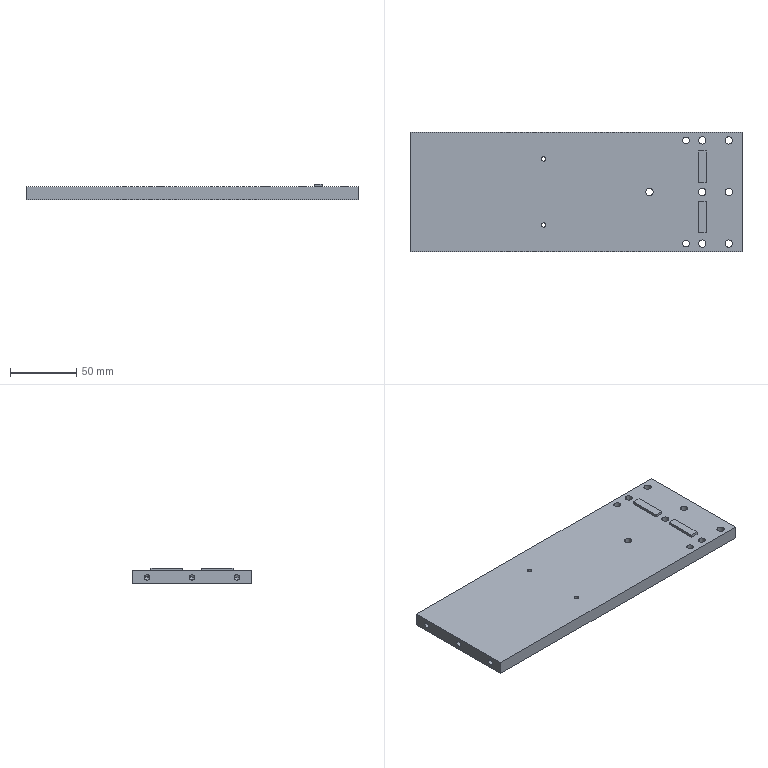CAM job | NX | 3-axis milling, drilling | part box 251 x 90 x 12 mm | stock box 257 x 94 x 13 mm
Tools:
number,name,description,diameter,corner_radius,flute_length,length,flutes
1,D63,Milling Tool-5 Parameters,63.0,0.0,50.0,75.0,2
10,D10,Milling Tool-5 Parameters,10.0,0.0,50.0,75.0,2
7,D6A45,Milling Tool-5 Parameters,6.0,0.0,3.0,3.0,2
16,5.5ZT,Drilling Tool,5.5,0.0,35.0,50.0,2
14,4.8ZT,Drilling Tool,4.8,0.0,35.0,50.0,2
15,5.0JD,Milling Tool-5 Parameters,5.0,0.0,30.0,30.0,4
13,3.3ZT,Drilling Tool,3.3,0.0,35.0,50.0,2
12,M4,Milling Tool-5 Parameters,3.3,0.0,30.0,30.0,4
11,D10JING,Milling Tool-5 Parameters,10.0,0.0,50.0,75.0,2
Operations:
program,operation,operation_type,tool,method,geometry_group,spindle_rpm,surface_speed,feed_per_tooth,feed_cut,feed_plunge,cut_length_mm,path_length_mm,cut_time_min,machine_time_min
1-254-90-15毛胚,FLOOR_WALL,VolumeBased25DMillingOperation,D63,METHOD,A,6500.0,1286.0,0.0962,1250.0,100.0,1040.797,1060.797,0.8326,0.8346
1-254-90-15毛胚,ADAPTIVE_MILLING,CavityMilling,D10,METHOD,A,7000.0,219.0,0.2143,3000.0,1000.0,26787.935,27444.133,8.937,9.003
1-254-90-15毛胚,DRILLING_COPY_1,Operation,D6A45,METHOD,A,3000.0,56.0,0.0333,200.0,0.0,56.1,554.367,0.2805,0.3303
1-254-90-15毛胚,DRILLING_COPY_1_COPY,Operation,5.5ZT,METHOD,A,2000.0,15.0,0.0375,150.0,0.0,107.667,492.181,0.7178,0.7562
1-254-90-15毛胚,DRILLING_COPY_1_COPY_COPY,Operation,4.8ZT,METHOD,A,2000.0,15.0,0.0375,150.0,0.0,31.884,208.826,0.2126,0.2303
1-254-90-15毛胚,DRILLING_COPY_1_COPY_COPY_COPY_COPY,Operation,5.0JD,METHOD,A,1000.0,15.0,0.0125,50.0,0.0,27.0,199.058,0.54,0.5572
1-254-90-15毛胚,DRILLING_COPY_1_COPY_COPY_COPY,Operation,3.3ZT,METHOD,A,1000.0,15.0,0.0125,50.0,0.0,30.983,179.056,0.6197,0.6345
1-254-90-15毛胚,DRILLING_COPY_1_COPY_COPY_COPY_COPY_1,Operation,M4,METHOD,A,200.0,2.0,0.175,140.0,0.0,27.0,171.09,0.1929,0.2073
1-254-90-15毛胚,ZLEVEL_PROFILE_COPY_COPY_1,ZLevelMilling,D10JING,METHOD,A,7000.0,219.0,0.0714,1000.0,100.0,725.308,771.308,0.7253,0.7299
1-254-90-15毛胚,FLOOR_WALL_1_COPY_1,VolumeBased25DMillingOperation,D10JING,METHOD,A,7000.0,87.0,0.0714,1000.0,100.0,5364.157,5783.12,5.364,5.426
1-254-90-15毛胚,ZLEVEL_PROFILE_COPY_1_COPY_COPY_COPY_COPY_2_COPY_COPY,ZLevelMilling,D6A45,METHOD,A,7000.0,131.0,0.0714,1000.0,1000.0,137.843,216.35,0.1378,0.1457
1-254-90-15毛胚,ZLEVEL_PROFILE_COPY_1_COPY_COPY_COPY_COPY_2_COPY_COPY_COPY,ZLevelMilling,D6A45,METHOD,A,7000.0,131.0,0.0714,1000.0,1000.0,830.386,2046.298,0.8304,0.952